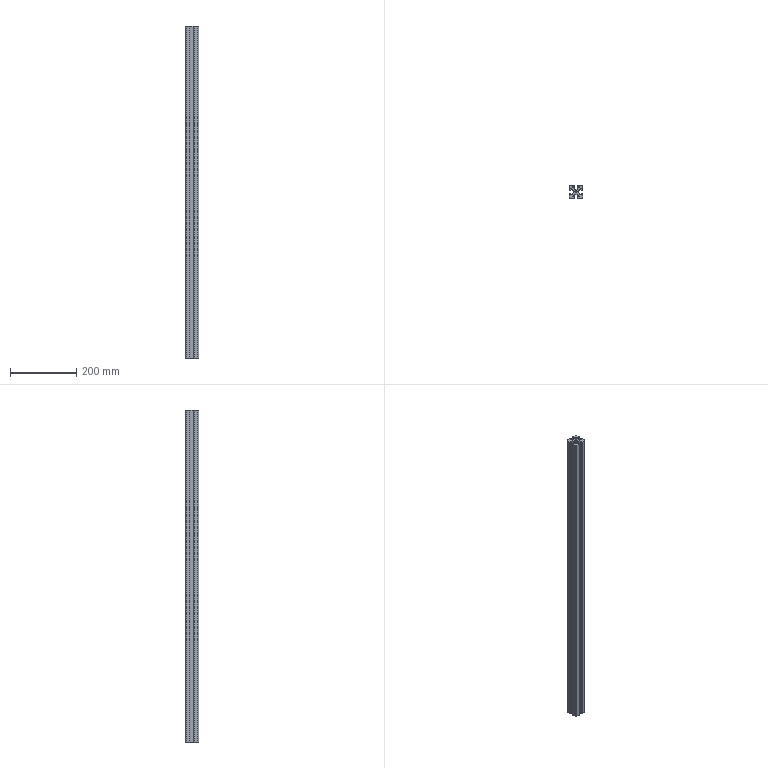Part | SolidWorks | features Extrusion 1 | 1 solid | 78 faces | box 40 x 40 x 1000 mm | volume 950664 mm3 | cylinder 48 | plane 30 | commonest cylinder face diameters 2 x26 4 x8 49.184 x8 8 x4 6.8 x2